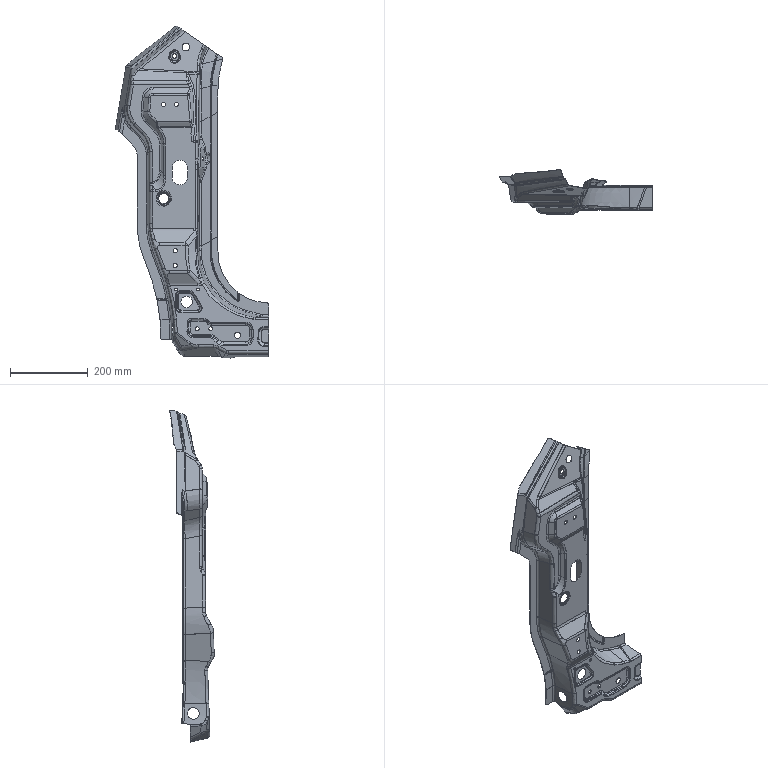Part | STEP file | FNA5401231 | 1 solid | 977 faces | box 393.159 x 114.364 x 853.043 mm | volume 316427 mm3 | spline 651 | cylinder 220 | plane 79 | other 15 | sphere 10 | torus 2 | commonest cylinder face diameters 10 x28 16 x23 13.6 x17 6 x14 7.6 x12 12.4 x12